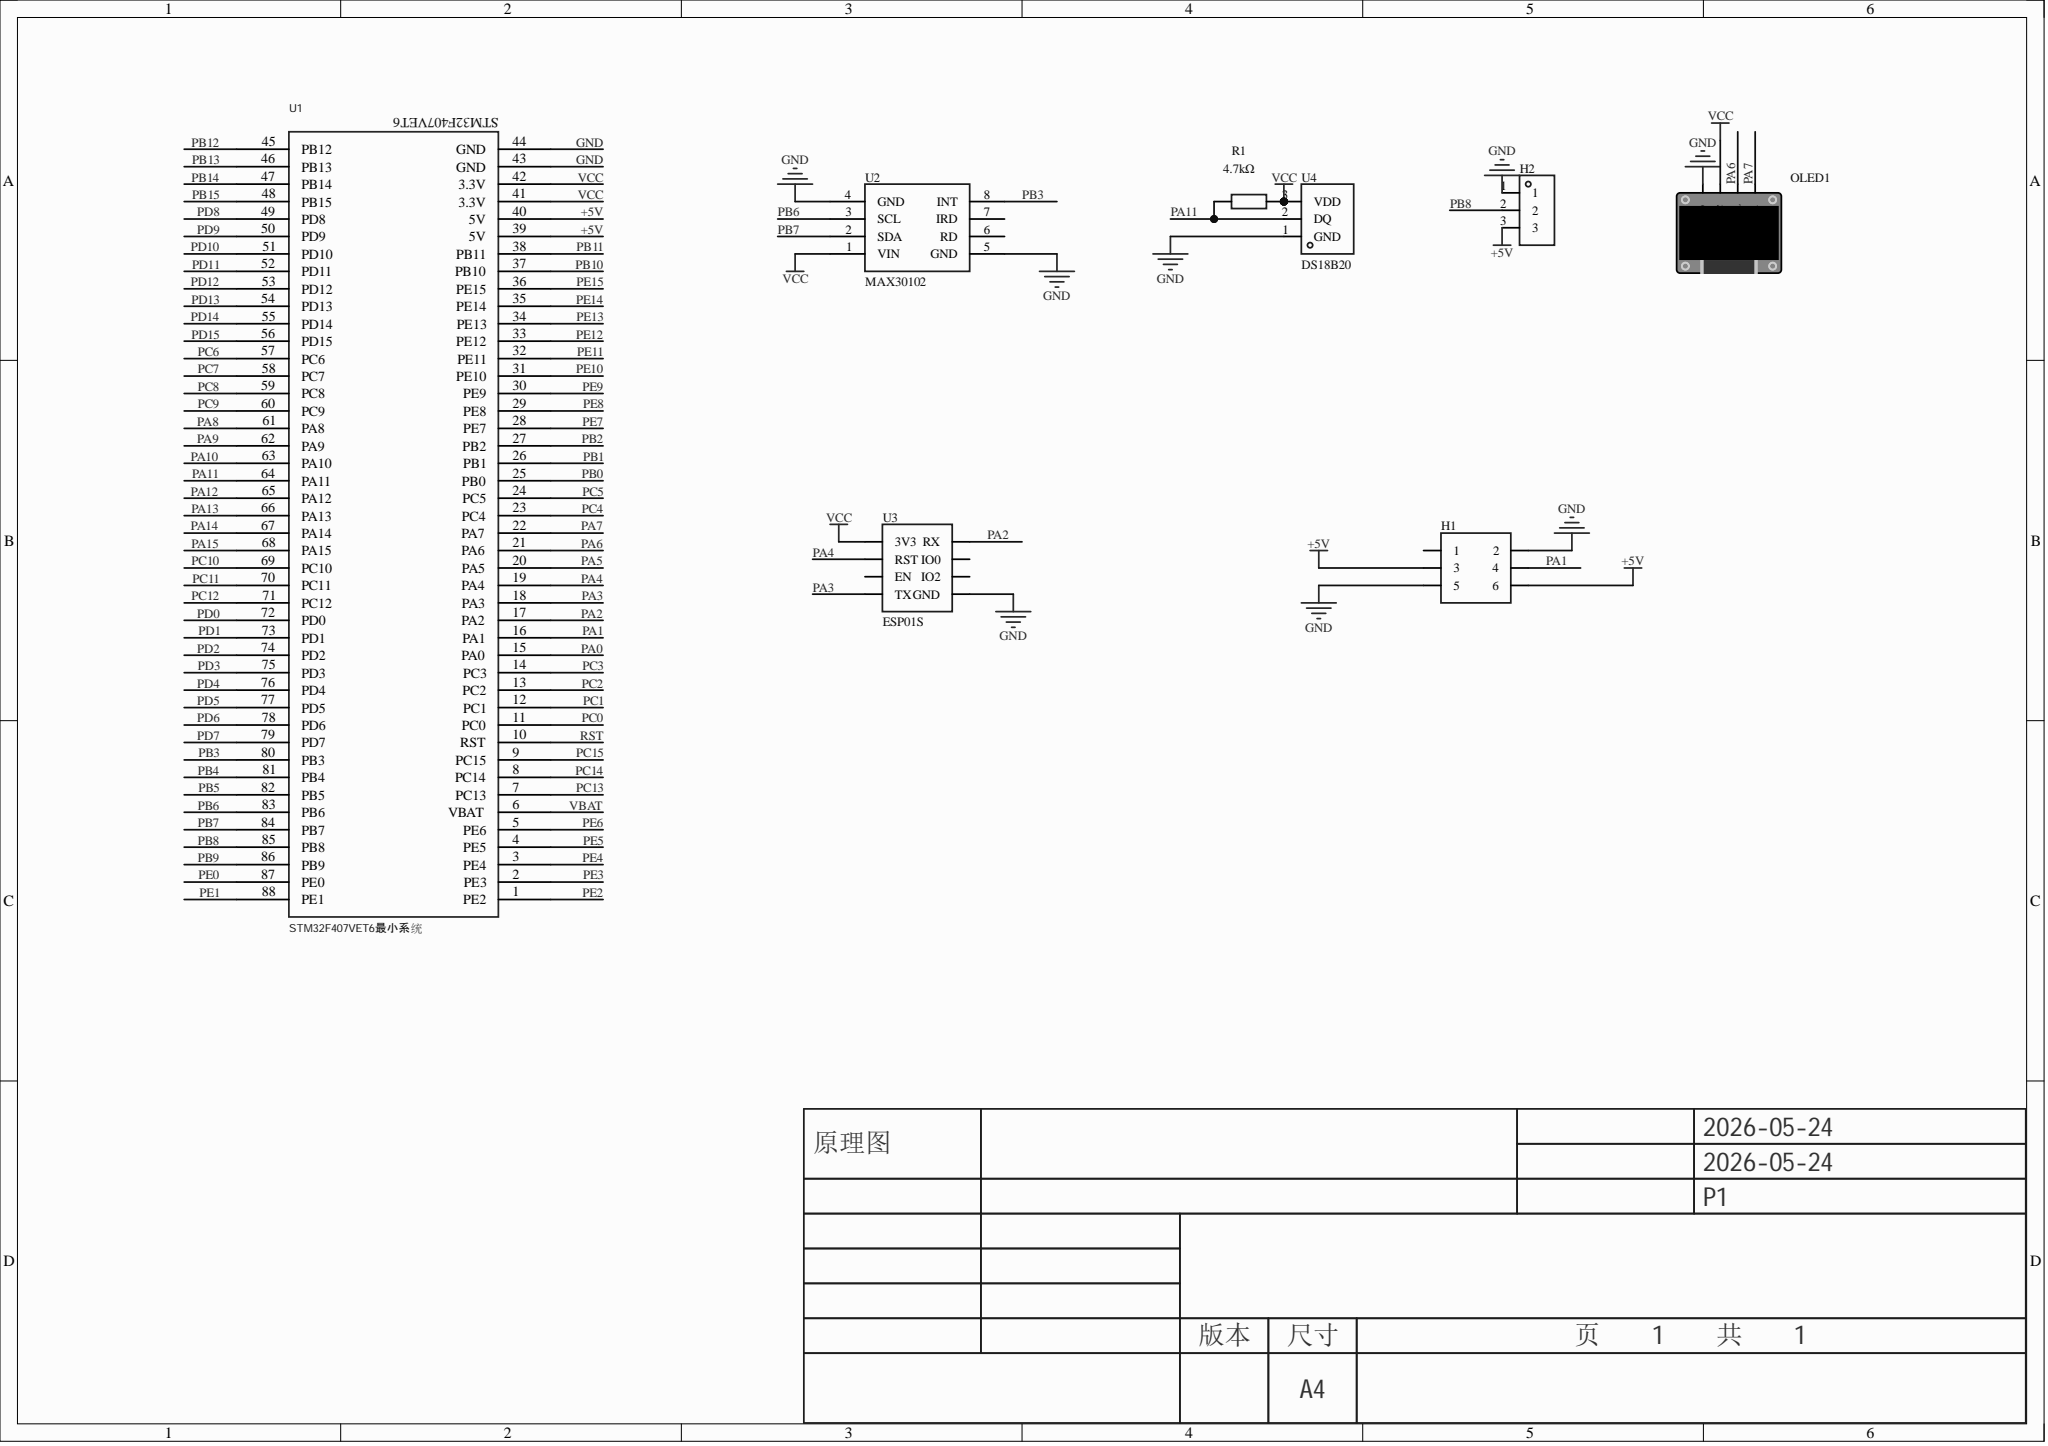Circuit board | Altium Designer | 8 parts | 14 nets
Bill of materials:
Comment,Description,Designator,Footprint,LibRef,Quantity
"","","H1","HDR-TH_6P-P2.54-V-F-R2-C3-S2.54","HDR-F_2.54_2x3","1"
"","","H2","HDR-TH_3P-P2.54-V-F","HDR-F_2.54_1x3P","1"
"","","OLED1","0.96OLED_4P","0.96OLED模块_4P","1"
"4.7kΩ","","R1","Res_1/8W","Res_AXIAL-1/8W","1"
"STM32F407VET6最小系统","","U1","STM32F407VET6最小系统","STM32F407VET6最小系统","1"
"MAX30102","","U2","MAX30102","MAX30102","1"
"ESP01S","","U3","ESP01S","ESP01S","1"
"DS18B20","检测温度:-55℃~+125℃;精度:±0.4℃;接口类型:单总线;","U4","TO-92-3_L4.5-W3.5-P1.27-L","DS18B20","1"
Netlist (Protel format):
[
H1
HDR-TH_6P-P2.54-V-F-R2-C3-S2.54




]
[
H2
HDR-TH_3P-P2.54-V-F




]
[
OLED1
0.96OLED_4P




]
[
R1
Res_1/8W
4.7kΩ



]
[
U1
STM32F407VET6最小系统
STM32F407VET6最小系统



]
[
U2
MAX30102
MAX30102



]
[
U3
ESP01S
ESP01S



]
[
U4
TO-92-3_L4.5-W3.5-P1.27-L
DS18B20



]
(
VCC
OLED1-2
R1-2
U1-41
U1-42
U2-1
U3-1
U4-3
)
(
PB8
H2-2
U1-85
)
(
PB7
U1-84
U2-2
)
(
PB6
U1-83
U2-3
)
(
PB3
U1-80
U2-8
)
(
PA11
R1-1
U1-64
U4-2
)
(
PA7
OLED1-4
U1-22
)
(
PA6
OLED1-3
U1-21
)
(
PA4
U1-19
U3-2
)
(
PA3
U1-18
U3-4
)
(
PA2
U1-17
U3-8
)
(
PA1
H1-4
U1-16
)
(
GND
H1-2
H1-5
H2-1
OLED1-1
U1-43
U1-44
U2-4
U2-5
U3-5
U4-1
)
(
+5V
H1-3
H1-6
H2-3
U1-39
U1-40
)